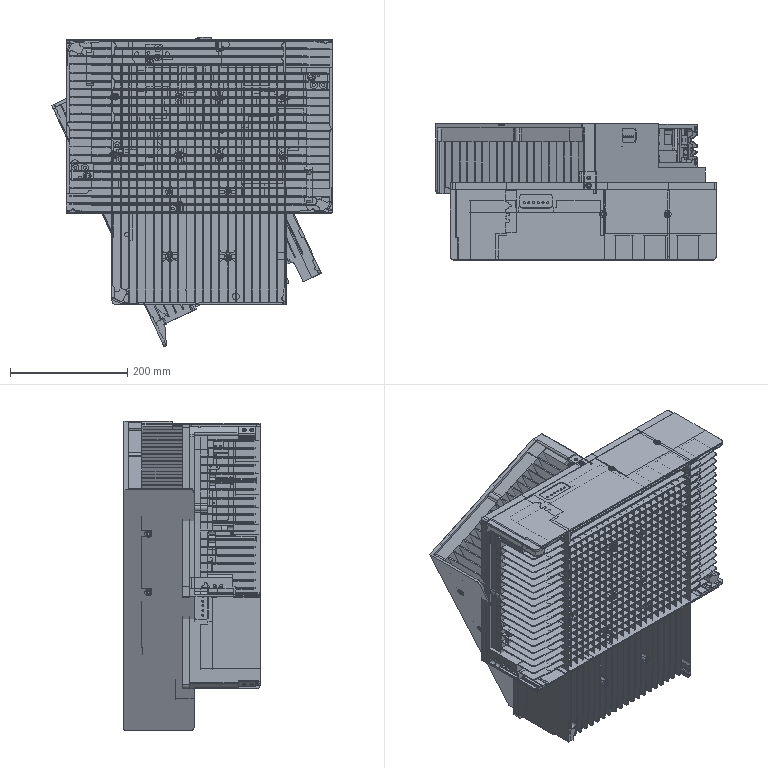Part | 17 solids | 19013 faces | volume 22880908 mm3 | plane 9740 | cylinder 6629 | spline 1366 | cone 1272 | torus 6 | commonest cylinder face diameters 2 x1105 6 x910 5 x810 10 x630 12 x499 3.3 x396